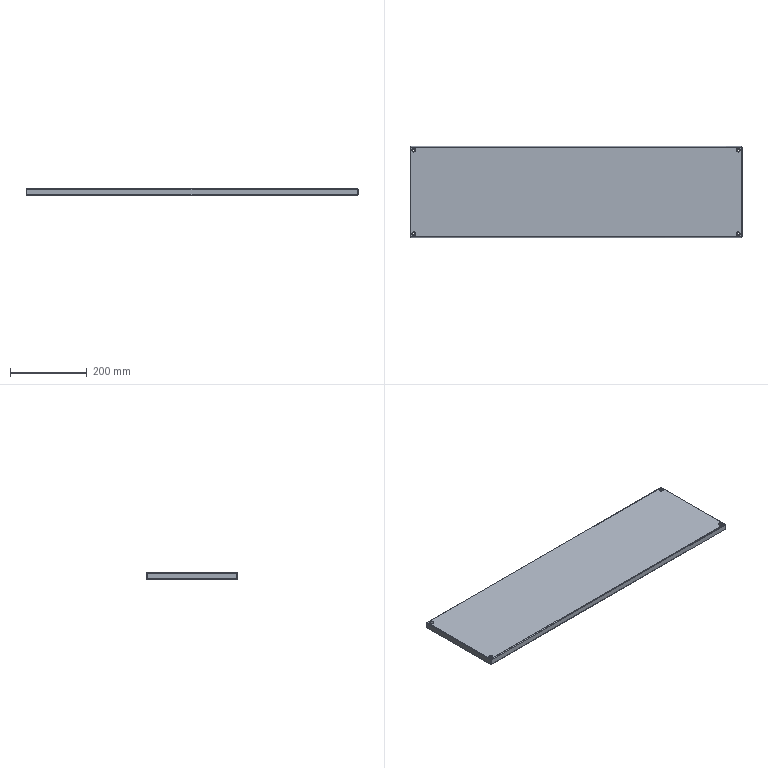Part | SolidWorks | features EdgeFlange 2, Cut 1, FlatPattern 1, HoleWzd 1, SMBaseFlange 1, SheetMetal 1 | 1 solid | 98 faces | box 868 x 238 x 17.5 mm | volume 401918 mm3 | plane 46 | cylinder 36 | spline 16 | commonest cylinder face diameters 5.8 x12 1 x8 4 x8 10 x8